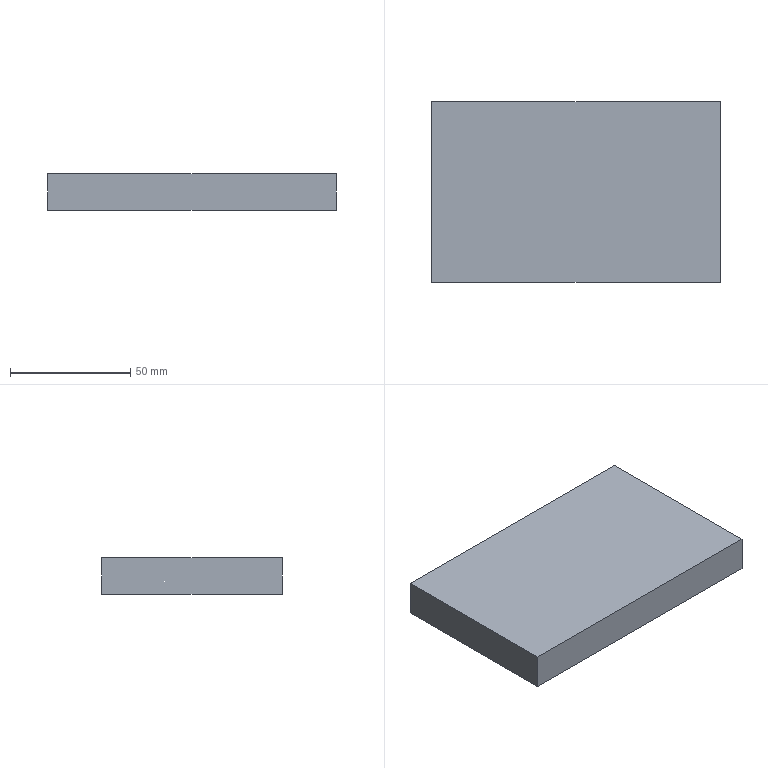Part | STEP file | Tube feed_id570_x_t | 1 solid | 6 faces | box 120 x 75 x 15 mm | volume 135000 mm3 | plane 6
STEP:
#1=CARTESIAN_POINT('',(0.,0.,0.));
#2=DIRECTION('',(0.,0.,1.));
#3=DIRECTION('',(1.,0.,0.));
#4=AXIS2_PLACEMENT_3D('',#1,#2,#3);
#5=CARTESIAN_POINT('',(496.,571.936,-204.));
#6=VERTEX_POINT('',#5);
#7=CARTESIAN_POINT('',(496.,496.936,-204.));
#8=VERTEX_POINT('',#7);
#9=CARTESIAN_POINT('',(496.,571.936,-204.));
#10=DIRECTION('',(0.,-1.,0.));
#11=VECTOR('',#10,1.);
#12=LINE('',#9,#11);
#13=CARTESIAN_POINT('',(496.,571.936,-219.));
#14=DIRECTION('',(-1.,0.,0.));
#15=DIRECTION('',(0.,-1.,0.));
#16=AXIS2_PLACEMENT_3D('',#13,#14,#15);
#17=PLANE('',#16);
#18=CARTESIAN_POINT('',(0.,15.));
#19=DIRECTION('',(1.,0.));
#20=VECTOR('',#19,1.);
#21=LINE('',#18,#20);
#22=(GEOMETRIC_REPRESENTATION_CONTEXT(2)PARAMETRIC_REPRESENTATION_CONTEXT()REPRESENTATION_CONTEXT('',''));
#23=DEFINITIONAL_REPRESENTATION('',(#21),#22);
#24=PCURVE('',#17,#23);
#25=CARTESIAN_POINT('',(0.,0.,-204.));
#26=DIRECTION('',(0.,0.,1.));
#27=DIRECTION('',(1.,0.,0.));
#28=AXIS2_PLACEMENT_3D('',#25,#26,#27);
#29=PLANE('',#28);
#30=CARTESIAN_POINT('',(496.,571.936));
#31=DIRECTION('',(0.,-1.));
#32=VECTOR('',#31,1.);
#33=LINE('',#30,#32);
#34=(GEOMETRIC_REPRESENTATION_CONTEXT(2)PARAMETRIC_REPRESENTATION_CONTEXT()REPRESENTATION_CONTEXT('',''));
#35=DEFINITIONAL_REPRESENTATION('',(#33),#34);
#36=PCURVE('',#29,#35);
#37=SURFACE_CURVE('',#12,(#24,#36),.PCURVE_S1.);
#38=EDGE_CURVE('',#6,#8,#37,.T.);
#39=ORIENTED_EDGE('',*,*,#38,.F.);
#40=CARTESIAN_POINT('',(496.,571.936,-219.));
#41=VERTEX_POINT('',#40);
#42=CARTESIAN_POINT('',(496.,571.936,-219.));
#43=DIRECTION('',(0.,0.,1.));
#44=VECTOR('',#43,1.);
#45=LINE('',#42,#44);
#46=CARTESIAN_POINT('',(0.,0.));
#47=DIRECTION('',(0.,1.));
#48=VECTOR('',#47,1.);
#49=LINE('',#46,#48);
#50=(GEOMETRIC_REPRESENTATION_CONTEXT(2)PARAMETRIC_REPRESENTATION_CONTEXT()REPRESENTATION_CONTEXT('',''));
#51=DEFINITIONAL_REPRESENTATION('',(#49),#50);
#52=PCURVE('',#17,#51);
#53=CARTESIAN_POINT('',(616.,571.936,-219.));
#54=DIRECTION('',(0.,1.,0.));
#55=DIRECTION('',(-1.,0.,0.));
#56=AXIS2_PLACEMENT_3D('',#53,#54,#55);
#57=PLANE('',#56);
#58=CARTESIAN_POINT('',(120.,0.));
#59=DIRECTION('',(0.,1.));
#60=VECTOR('',#59,1.);
#61=LINE('',#58,#60);
#62=(GEOMETRIC_REPRESENTATION_CONTEXT(2)PARAMETRIC_REPRESENTATION_CONTEXT()REPRESENTATION_CONTEXT('',''));
#63=DEFINITIONAL_REPRESENTATION('',(#61),#62);
#64=PCURVE('',#57,#63);
#65=SURFACE_CURVE('',#45,(#52,#64),.PCURVE_S1.);
#66=EDGE_CURVE('',#41,#6,#65,.T.);
#67=ORIENTED_EDGE('',*,*,#66,.F.);
#68=CARTESIAN_POINT('',(496.,496.936,-219.));
#69=VERTEX_POINT('',#68);
#70=CARTESIAN_POINT('',(496.,571.936,-219.));
#71=DIRECTION('',(0.,-1.,0.));
#72=VECTOR('',#71,1.);
#73=LINE('',#70,#72);
#74=CARTESIAN_POINT('',(0.,0.));
#75=DIRECTION('',(1.,0.));
#76=VECTOR('',#75,1.);
#77=LINE('',#74,#76);
#78=(GEOMETRIC_REPRESENTATION_CONTEXT(2)PARAMETRIC_REPRESENTATION_CONTEXT()REPRESENTATION_CONTEXT('',''));
#79=DEFINITIONAL_REPRESENTATION('',(#77),#78);
#80=PCURVE('',#17,#79);
#81=CARTESIAN_POINT('',(0.,0.,-219.));
#82=DIRECTION('',(0.,0.,1.));
#83=DIRECTION('',(1.,0.,0.));
#84=AXIS2_PLACEMENT_3D('',#81,#82,#83);
#85=PLANE('',#84);
#86=CARTESIAN_POINT('',(496.,571.936));
#87=DIRECTION('',(0.,-1.));
#88=VECTOR('',#87,1.);
#89=LINE('',#86,#88);
#90=(GEOMETRIC_REPRESENTATION_CONTEXT(2)PARAMETRIC_REPRESENTATION_CONTEXT()REPRESENTATION_CONTEXT('',''));
#91=DEFINITIONAL_REPRESENTATION('',(#89),#90);
#92=PCURVE('',#85,#91);
#93=SURFACE_CURVE('',#73,(#80,#92),.PCURVE_S1.);
#94=EDGE_CURVE('',#41,#69,#93,.T.);
#95=ORIENTED_EDGE('',*,*,#94,.T.);
#96=CARTESIAN_POINT('',(496.,496.936,-219.));
#97=DIRECTION('',(0.,0.,1.));
#98=VECTOR('',#97,1.);
#99=LINE('',#96,#98);
#100=CARTESIAN_POINT('',(75.,0.));
#101=DIRECTION('',(0.,1.));
#102=VECTOR('',#101,1.);
#103=LINE('',#100,#102);
#104=(GEOMETRIC_REPRESENTATION_CONTEXT(2)PARAMETRIC_REPRESENTATION_CONTEXT()REPRESENTATION_CONTEXT('',''));
#105=DEFINITIONAL_REPRESENTATION('',(#103),#104);
#106=PCURVE('',#17,#105);
#107=CARTESIAN_POINT('',(496.,496.936,-219.));
#108=DIRECTION('',(0.,-1.,0.));
#109=DIRECTION('',(0.,0.,-1.));
#110=AXIS2_PLACEMENT_3D('',#107,#108,#109);
#111=PLANE('',#110);
#112=CARTESIAN_POINT('',(0.,0.));
#113=DIRECTION('',(-1.,0.));
#114=VECTOR('',#113,1.);
#115=LINE('',#112,#114);
#116=(GEOMETRIC_REPRESENTATION_CONTEXT(2)PARAMETRIC_REPRESENTATION_CONTEXT()REPRESENTATION_CONTEXT('',''));
#117=DEFINITIONAL_REPRESENTATION('',(#115),#116);
#118=PCURVE('',#111,#117);
#119=SURFACE_CURVE('',#99,(#106,#118),.PCURVE_S1.);
#120=EDGE_CURVE('',#69,#8,#119,.T.);
#121=ORIENTED_EDGE('',*,*,#120,.T.);
#122=EDGE_LOOP('',(#39,#67,#95,#121));
#123=FACE_BOUND('',#122,.T.);
#124=ADVANCED_FACE('',(#123),#17,.T.);
#125=CARTESIAN_POINT('',(616.,496.936,-204.));
#126=VERTEX_POINT('',#125);
#127=CARTESIAN_POINT('',(496.,496.936,-204.));
#128=DIRECTION('',(1.,0.,0.));
#129=VECTOR('',#128,1.);
#130=LINE('',#127,#129);
#131=CARTESIAN_POINT('',(-15.,0.));
#132=DIRECTION('',(0.,1.));
#133=VECTOR('',#132,1.);
#134=LINE('',#131,#133);
#135=(GEOMETRIC_REPRESENTATION_CONTEXT(2)PARAMETRIC_REPRESENTATION_CONTEXT()REPRESENTATION_CONTEXT('',''));
#136=DEFINITIONAL_REPRESENTATION('',(#134),#135);
#137=PCURVE('',#111,#136);
#138=CARTESIAN_POINT('',(496.,496.936));
#139=DIRECTION('',(1.,0.));
#140=VECTOR('',#139,1.);
#141=LINE('',#138,#140);
#142=(GEOMETRIC_REPRESENTATION_CONTEXT(2)PARAMETRIC_REPRESENTATION_CONTEXT()REPRESENTATION_CONTEXT('',''));
#143=DEFINITIONAL_REPRESENTATION('',(#141),#142);
#144=PCURVE('',#29,#143);
#145=SURFACE_CURVE('',#130,(#137,#144),.PCURVE_S1.);
#146=EDGE_CURVE('',#8,#126,#145,.T.);
#147=ORIENTED_EDGE('',*,*,#146,.F.);
#148=ORIENTED_EDGE('',*,*,#120,.F.);
#149=CARTESIAN_POINT('',(616.,496.936,-219.));
#150=VERTEX_POINT('',#149);
#151=CARTESIAN_POINT('',(496.,496.936,-219.));
#152=DIRECTION('',(1.,0.,0.));
#153=VECTOR('',#152,1.);
#154=LINE('',#151,#153);
#155=CARTESIAN_POINT('',(0.,0.));
#156=DIRECTION('',(0.,1.));
#157=VECTOR('',#156,1.);
#158=LINE('',#155,#157);
#159=(GEOMETRIC_REPRESENTATION_CONTEXT(2)PARAMETRIC_REPRESENTATION_CONTEXT()REPRESENTATION_CONTEXT('',''));
#160=DEFINITIONAL_REPRESENTATION('',(#158),#159);
#161=PCURVE('',#111,#160);
#162=CARTESIAN_POINT('',(496.,496.936));
#163=DIRECTION('',(1.,0.));
#164=VECTOR('',#163,1.);
#165=LINE('',#162,#164);
#166=(GEOMETRIC_REPRESENTATION_CONTEXT(2)PARAMETRIC_REPRESENTATION_CONTEXT()REPRESENTATION_CONTEXT('',''));
#167=DEFINITIONAL_REPRESENTATION('',(#165),#166);
#168=PCURVE('',#85,#167);
#169=SURFACE_CURVE('',#154,(#161,#168),.PCURVE_S1.);
#170=EDGE_CURVE('',#69,#150,#169,.T.);
#171=ORIENTED_EDGE('',*,*,#170,.T.);
#172=CARTESIAN_POINT('',(616.,496.936,-219.));
#173=DIRECTION('',(0.,0.,1.));
#174=VECTOR('',#173,1.);
#175=LINE('',#172,#174);
#176=CARTESIAN_POINT('',(0.,120.));
#177=DIRECTION('',(-1.,0.));
#178=VECTOR('',#177,1.);
#179=LINE('',#176,#178);
#180=(GEOMETRIC_REPRESENTATION_CONTEXT(2)PARAMETRIC_REPRESENTATION_CONTEXT()REPRESENTATION_CONTEXT('',''));
#181=DEFINITIONAL_REPRESENTATION('',(#179),#180);
#182=PCURVE('',#111,#181);
#183=CARTESIAN_POINT('',(616.,496.936,-219.));
#184=DIRECTION('',(1.,0.,0.));
#185=DIRECTION('',(0.,0.,-1.));
#186=AXIS2_PLACEMENT_3D('',#183,#184,#185);
#187=PLANE('',#186);
#188=CARTESIAN_POINT('',(0.,0.));
#189=DIRECTION('',(-1.,0.));
#190=VECTOR('',#189,1.);
#191=LINE('',#188,#190);
#192=(GEOMETRIC_REPRESENTATION_CONTEXT(2)PARAMETRIC_REPRESENTATION_CONTEXT()REPRESENTATION_CONTEXT('',''));
#193=DEFINITIONAL_REPRESENTATION('',(#191),#192);
#194=PCURVE('',#187,#193);
#195=SURFACE_CURVE('',#175,(#182,#194),.PCURVE_S1.);
#196=EDGE_CURVE('',#150,#126,#195,.T.);
#197=ORIENTED_EDGE('',*,*,#196,.T.);
#198=EDGE_LOOP('',(#147,#148,#171,#197));
#199=FACE_BOUND('',#198,.T.);
#200=ADVANCED_FACE('',(#199),#111,.T.);
#201=CARTESIAN_POINT('',(616.,571.936,-204.));
#202=VERTEX_POINT('',#201);
#203=CARTESIAN_POINT('',(616.,496.936,-204.));
#204=DIRECTION('',(0.,1.,0.));
#205=VECTOR('',#204,1.);
#206=LINE('',#203,#205);
#207=CARTESIAN_POINT('',(-15.,0.));
#208=DIRECTION('',(0.,1.));
#209=VECTOR('',#208,1.);
#210=LINE('',#207,#209);
#211=(GEOMETRIC_REPRESENTATION_CONTEXT(2)PARAMETRIC_REPRESENTATION_CONTEXT()REPRESENTATION_CONTEXT('',''));
#212=DEFINITIONAL_REPRESENTATION('',(#210),#211);
#213=PCURVE('',#187,#212);
#214=CARTESIAN_POINT('',(616.,496.936));
#215=DIRECTION('',(0.,1.));
#216=VECTOR('',#215,1.);
#217=LINE('',#214,#216);
#218=(GEOMETRIC_REPRESENTATION_CONTEXT(2)PARAMETRIC_REPRESENTATION_CONTEXT()REPRESENTATION_CONTEXT('',''));
#219=DEFINITIONAL_REPRESENTATION('',(#217),#218);
#220=PCURVE('',#29,#219);
#221=SURFACE_CURVE('',#206,(#213,#220),.PCURVE_S1.);
#222=EDGE_CURVE('',#126,#202,#221,.T.);
#223=ORIENTED_EDGE('',*,*,#222,.F.);
#224=ORIENTED_EDGE('',*,*,#196,.F.);
#225=CARTESIAN_POINT('',(616.,571.936,-219.));
#226=VERTEX_POINT('',#225);
#227=CARTESIAN_POINT('',(616.,496.936,-219.));
#228=DIRECTION('',(0.,1.,0.));
#229=VECTOR('',#228,1.);
#230=LINE('',#227,#229);
#231=CARTESIAN_POINT('',(0.,0.));
#232=DIRECTION('',(0.,1.));
#233=VECTOR('',#232,1.);
#234=LINE('',#231,#233);
#235=(GEOMETRIC_REPRESENTATION_CONTEXT(2)PARAMETRIC_REPRESENTATION_CONTEXT()REPRESENTATION_CONTEXT('',''));
#236=DEFINITIONAL_REPRESENTATION('',(#234),#235);
#237=PCURVE('',#187,#236);
#238=CARTESIAN_POINT('',(616.,496.936));
#239=DIRECTION('',(0.,1.));
#240=VECTOR('',#239,1.);
#241=LINE('',#238,#240);
#242=(GEOMETRIC_REPRESENTATION_CONTEXT(2)PARAMETRIC_REPRESENTATION_CONTEXT()REPRESENTATION_CONTEXT('',''));
#243=DEFINITIONAL_REPRESENTATION('',(#241),#242);
#244=PCURVE('',#85,#243);
#245=SURFACE_CURVE('',#230,(#237,#244),.PCURVE_S1.);
#246=EDGE_CURVE('',#150,#226,#245,.T.);
#247=ORIENTED_EDGE('',*,*,#246,.T.);
#248=CARTESIAN_POINT('',(616.,571.936,-219.));
#249=DIRECTION('',(0.,0.,1.));
#250=VECTOR('',#249,1.);
#251=LINE('',#248,#250);
#252=CARTESIAN_POINT('',(0.,75.));
#253=DIRECTION('',(-1.,0.));
#254=VECTOR('',#253,1.);
#255=LINE('',#252,#254);
#256=(GEOMETRIC_REPRESENTATION_CONTEXT(2)PARAMETRIC_REPRESENTATION_CONTEXT()REPRESENTATION_CONTEXT('',''));
#257=DEFINITIONAL_REPRESENTATION('',(#255),#256);
#258=PCURVE('',#187,#257);
#259=CARTESIAN_POINT('',(0.,0.));
#260=DIRECTION('',(0.,1.));
#261=VECTOR('',#260,1.);
#262=LINE('',#259,#261);
#263=(GEOMETRIC_REPRESENTATION_CONTEXT(2)PARAMETRIC_REPRESENTATION_CONTEXT()REPRESENTATION_CONTEXT('',''));
#264=DEFINITIONAL_REPRESENTATION('',(#262),#263);
#265=PCURVE('',#57,#264);
#266=SURFACE_CURVE('',#251,(#258,#265),.PCURVE_S1.);
#267=EDGE_CURVE('',#226,#202,#266,.T.);
#268=ORIENTED_EDGE('',*,*,#267,.T.);
#269=EDGE_LOOP('',(#223,#224,#247,#268));
#270=FACE_BOUND('',#269,.T.);
#271=ADVANCED_FACE('',(#270),#187,.T.);
#272=CARTESIAN_POINT('',(616.,571.936,-204.));
#273=DIRECTION('',(-1.,0.,0.));
#274=VECTOR('',#273,1.);
#275=LINE('',#272,#274);
#276=CARTESIAN_POINT('',(0.,15.));
#277=DIRECTION('',(1.,0.));
#278=VECTOR('',#277,1.);
#279=LINE('',#276,#278);
#280=(GEOMETRIC_REPRESENTATION_CONTEXT(2)PARAMETRIC_REPRESENTATION_CONTEXT()REPRESENTATION_CONTEXT('',''));
#281=DEFINITIONAL_REPRESENTATION('',(#279),#280);
#282=PCURVE('',#57,#281);
#283=CARTESIAN_POINT('',(616.,571.936));
#284=DIRECTION('',(-1.,0.));
#285=VECTOR('',#284,1.);
#286=LINE('',#283,#285);
#287=(GEOMETRIC_REPRESENTATION_CONTEXT(2)PARAMETRIC_REPRESENTATION_CONTEXT()REPRESENTATION_CONTEXT('',''));
#288=DEFINITIONAL_REPRESENTATION('',(#286),#287);
#289=PCURVE('',#29,#288);
#290=SURFACE_CURVE('',#275,(#282,#289),.PCURVE_S1.);
#291=EDGE_CURVE('',#202,#6,#290,.T.);
#292=ORIENTED_EDGE('',*,*,#291,.F.);
#293=ORIENTED_EDGE('',*,*,#267,.F.);
#294=CARTESIAN_POINT('',(616.,571.936,-219.));
#295=DIRECTION('',(-1.,0.,0.));
#296=VECTOR('',#295,1.);
#297=LINE('',#294,#296);
#298=CARTESIAN_POINT('',(0.,0.));
#299=DIRECTION('',(1.,0.));
#300=VECTOR('',#299,1.);
#301=LINE('',#298,#300);
#302=(GEOMETRIC_REPRESENTATION_CONTEXT(2)PARAMETRIC_REPRESENTATION_CONTEXT()REPRESENTATION_CONTEXT('',''));
#303=DEFINITIONAL_REPRESENTATION('',(#301),#302);
#304=PCURVE('',#57,#303);
#305=CARTESIAN_POINT('',(616.,571.936));
#306=DIRECTION('',(-1.,0.));
#307=VECTOR('',#306,1.);
#308=LINE('',#305,#307);
#309=(GEOMETRIC_REPRESENTATION_CONTEXT(2)PARAMETRIC_REPRESENTATION_CONTEXT()REPRESENTATION_CONTEXT('',''));
#310=DEFINITIONAL_REPRESENTATION('',(#308),#309);
#311=PCURVE('',#85,#310);
#312=SURFACE_CURVE('',#297,(#304,#311),.PCURVE_S1.);
#313=EDGE_CURVE('',#226,#41,#312,.T.);
#314=ORIENTED_EDGE('',*,*,#313,.T.);
#315=ORIENTED_EDGE('',*,*,#66,.T.);
#316=EDGE_LOOP('',(#292,#293,#314,#315));
#317=FACE_BOUND('',#316,.T.);
#318=ADVANCED_FACE('',(#317),#57,.T.);
#319=ORIENTED_EDGE('',*,*,#94,.F.);
#320=ORIENTED_EDGE('',*,*,#313,.F.);
#321=ORIENTED_EDGE('',*,*,#246,.F.);
#322=ORIENTED_EDGE('',*,*,#170,.F.);
#323=EDGE_LOOP('',(#319,#320,#321,#322));
#324=FACE_BOUND('',#323,.T.);
#325=ADVANCED_FACE('',(#324),#85,.F.);
#326=ORIENTED_EDGE('',*,*,#38,.T.);
#327=ORIENTED_EDGE('',*,*,#146,.T.);
#328=ORIENTED_EDGE('',*,*,#222,.T.);
#329=ORIENTED_EDGE('',*,*,#291,.T.);
#330=EDGE_LOOP('',(#326,#327,#328,#329));
#331=FACE_BOUND('',#330,.T.);
#332=ADVANCED_FACE('',(#331),#29,.T.);
#333=CLOSED_SHELL('',(#124,#200,#271,#318,#325,#332));
#334=MANIFOLD_SOLID_BREP('',#333);
#335=(LENGTH_UNIT()NAMED_UNIT(*)SI_UNIT(.MILLI.,.METRE.));
#336=UNCERTAINTY_MEASURE_WITH_UNIT(LENGTH_MEASURE(0.0000001),#335,'','');
#337=(NAMED_UNIT(*)PLANE_ANGLE_UNIT()SI_UNIT($,.RADIAN.));
#338=(NAMED_UNIT(*)SI_UNIT($,.STERADIAN.)SOLID_ANGLE_UNIT());
#339=(GEOMETRIC_REPRESENTATION_CONTEXT(3)GLOBAL_UNCERTAINTY_ASSIGNED_CONTEXT((#336))GLOBAL_UNIT_ASSIGNED_CONTEXT((#335,#337,#338))REPRESENTATION_CONTEXT('',''));
#340=ADVANCED_BREP_SHAPE_REPRESENTATION('',(#4,#334),#339);